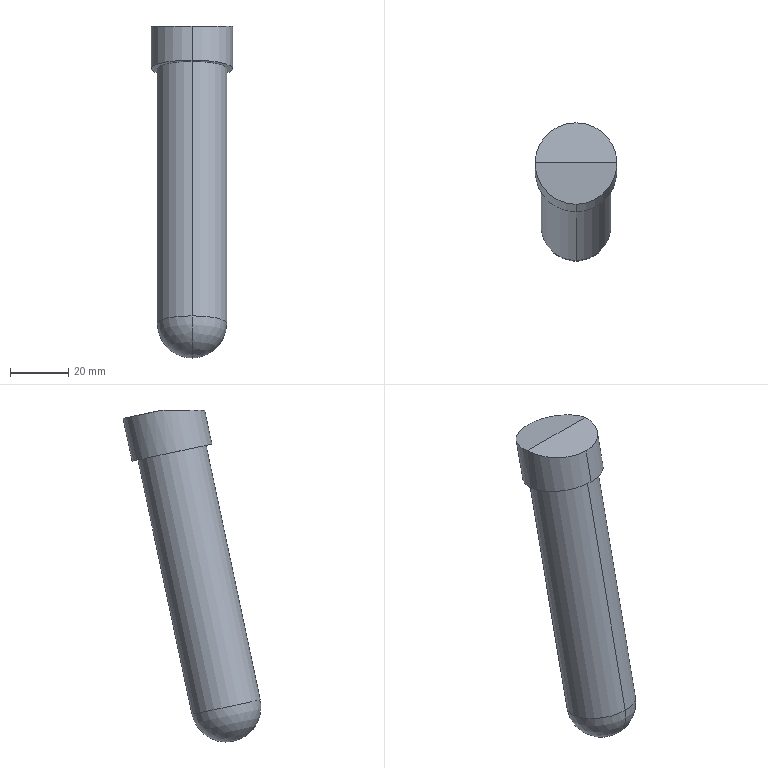Part | Creo | 1 solid | 9 faces | box 28.1 x 47.494 x 114.331 mm | volume 53070 mm3 | cylinder 4 | plane 3 | sphere 2 | commonest cylinder face diameters 24 x2 28.1 x2
STEP:
#1=CARTESIAN_POINT('',(110.,-266.619,89.579));
#2=VERTEX_POINT('',#1);
#3=CARTESIAN_POINT('',(95.95,-280.362,92.5));
#4=VERTEX_POINT('',#3);
#5=CARTESIAN_POINT('',(110.,-280.362,92.5));
#6=DIRECTION('',(0.,0.2079,0.9781));
#7=DIRECTION('',(0.,0.9781,-0.2079));
#8=AXIS2_PLACEMENT_3D('',#5,#6,#7);
#9=CIRCLE('',#8,14.05);
#10=EDGE_CURVE('',#2,#4,#9,.T.);
#11=ORIENTED_EDGE('',*,*,#10,.F.);
#12=CARTESIAN_POINT('',(124.05,-280.362,92.5));
#13=VERTEX_POINT('',#12);
#14=CARTESIAN_POINT('',(110.,-280.362,92.5));
#15=DIRECTION('',(0.,0.2079,0.9781));
#16=DIRECTION('',(1.,0.,0.));
#17=AXIS2_PLACEMENT_3D('',#14,#15,#16);
#18=CIRCLE('',#17,14.05);
#19=EDGE_CURVE('',#13,#2,#18,.T.);
#20=ORIENTED_EDGE('',*,*,#19,.F.);
#21=CARTESIAN_POINT('',(95.95,-280.362,92.5));
#22=DIRECTION('',(1.,0.,0.));
#23=VECTOR('',#22,28.1);
#24=LINE('',#21,#23);
#25=EDGE_CURVE('',#4,#13,#24,.T.);
#26=ORIENTED_EDGE('',*,*,#25,.F.);
#27=EDGE_LOOP('',(#11,#20,#26));
#28=FACE_OUTER_BOUND('',#27,.F.);
#29=CARTESIAN_POINT('',(110.,-280.362,92.5));
#30=DIRECTION('',(0.,0.2079,0.9781));
#31=DIRECTION('',(0.,-0.9781,0.2079));
#32=AXIS2_PLACEMENT_3D('',#29,#30,#31);
#33=PLANE('',#32);
#34=ADVANCED_FACE('',(#28),#33,.T.);
#35=CARTESIAN_POINT('',(110.,-297.224,80.749));
#36=VERTEX_POINT('',#35);
#37=CARTESIAN_POINT('',(110.,-269.738,74.907));
#38=VERTEX_POINT('',#37);
#39=CARTESIAN_POINT('',(110.,-283.481,77.828));
#40=DIRECTION('',(0.,-0.2079,-0.9781));
#41=DIRECTION('',(0.,-0.9781,0.2079));
#42=AXIS2_PLACEMENT_3D('',#39,#40,#41);
#43=CIRCLE('',#42,14.05);
#44=EDGE_CURVE('',#36,#38,#43,.T.);
#45=ORIENTED_EDGE('',*,*,#44,.T.);
#46=CARTESIAN_POINT('',(110.,-266.619,89.579));
#47=DIRECTION('',(0.,-0.2079,-0.9781));
#48=VECTOR('',#47,15.);
#49=LINE('',#46,#48);
#50=EDGE_CURVE('',#2,#38,#49,.T.);
#51=ORIENTED_EDGE('',*,*,#50,.F.);
#52=ORIENTED_EDGE('',*,*,#10,.T.);
#53=CARTESIAN_POINT('',(110.,-294.726,92.5));
#54=VERTEX_POINT('',#53);
#55=CARTESIAN_POINT('',(110.,-294.726,92.5));
#56=CARTESIAN_POINT('',(109.185,-294.726,92.5));
#57=CARTESIAN_POINT('',(107.581,-294.584,92.5));
#58=CARTESIAN_POINT('',(105.216,-293.946,92.5));
#59=CARTESIAN_POINT('',(102.983,-292.89,92.5));
#60=CARTESIAN_POINT('',(100.982,-291.47,92.5));
#61=CARTESIAN_POINT('',(99.234,-289.706,92.5));
#62=CARTESIAN_POINT('',(97.802,-287.636,92.5));
#63=CARTESIAN_POINT('',(96.753,-285.365,92.5));
#64=CARTESIAN_POINT('',(96.099,-282.91,92.5));
#65=CARTESIAN_POINT('',(95.95,-281.224,92.5));
#66=CARTESIAN_POINT('',(95.95,-280.362,92.5));
#67=B_SPLINE_CURVE_WITH_KNOTS('',3,(#55,#56,#57,#58,#59,#60,#61,#62,#63,#64,#65,#66),.UNSPECIFIED.,.F.,.F.,(4,1,1,1,1,1,1,1,1,4),(0.,0.1111,0.2222,0.3333,0.4444,0.5556,0.6667,0.7778,0.8889,1.),.UNSPECIFIED.);
#68=EDGE_CURVE('',#54,#4,#67,.T.);
#69=ORIENTED_EDGE('',*,*,#68,.F.);
#70=CARTESIAN_POINT('',(110.,-294.726,92.5));
#71=DIRECTION('',(0.,-0.2079,-0.9781));
#72=VECTOR('',#71,12.014);
#73=LINE('',#70,#72);
#74=EDGE_CURVE('',#54,#36,#73,.T.);
#75=ORIENTED_EDGE('',*,*,#74,.T.);
#76=EDGE_LOOP('',(#45,#51,#52,#69,#75));
#77=FACE_OUTER_BOUND('',#76,.F.);
#78=CARTESIAN_POINT('',(110.,-280.362,92.5));
#79=DIRECTION('',(0.,-0.2079,-0.9781));
#80=DIRECTION('',(0.,0.9781,-0.2079));
#81=AXIS2_PLACEMENT_3D('',#78,#79,#80);
#82=CYLINDRICAL_SURFACE('',#81,14.05);
#83=ADVANCED_FACE('',(#77),#82,.T.);
#84=ORIENTED_EDGE('',*,*,#44,.F.);
#85=CARTESIAN_POINT('',(110.,-283.481,77.828));
#86=DIRECTION('',(0.,-0.2079,-0.9781));
#87=DIRECTION('',(0.,0.9781,-0.2079));
#88=AXIS2_PLACEMENT_3D('',#85,#86,#87);
#89=CIRCLE('',#88,14.05);
#90=EDGE_CURVE('',#38,#36,#89,.T.);
#91=ORIENTED_EDGE('',*,*,#90,.F.);
#92=EDGE_LOOP('',(#84,#91));
#93=FACE_OUTER_BOUND('',#92,.F.);
#94=CARTESIAN_POINT('',(110.,-271.743,75.333));
#95=VERTEX_POINT('',#94);
#96=CARTESIAN_POINT('',(110.,-295.219,80.323));
#97=VERTEX_POINT('',#96);
#98=CARTESIAN_POINT('',(110.,-283.481,77.828));
#99=DIRECTION('',(0.,0.2079,0.9781));
#100=DIRECTION('',(0.,0.9781,-0.2079));
#101=AXIS2_PLACEMENT_3D('',#98,#99,#100);
#102=CIRCLE('',#101,12.);
#103=EDGE_CURVE('',#95,#97,#102,.T.);
#104=ORIENTED_EDGE('',*,*,#103,.F.);
#105=CARTESIAN_POINT('',(110.,-283.481,77.828));
#106=DIRECTION('',(0.,0.2079,0.9781));
#107=DIRECTION('',(0.,-0.9781,0.2079));
#108=AXIS2_PLACEMENT_3D('',#105,#106,#107);
#109=CIRCLE('',#108,12.);
#110=EDGE_CURVE('',#97,#95,#109,.T.);
#111=ORIENTED_EDGE('',*,*,#110,.F.);
#112=EDGE_LOOP('',(#104,#111));
#113=FACE_BOUND('',#112,.F.);
#114=CARTESIAN_POINT('',(110.,-283.481,77.828));
#115=DIRECTION('',(0.,-0.2079,-0.9781));
#116=DIRECTION('',(0.,0.9781,-0.2079));
#117=AXIS2_PLACEMENT_3D('',#114,#115,#116);
#118=PLANE('',#117);
#119=ADVANCED_FACE('',(#93,#113),#118,.T.);
#120=ORIENTED_EDGE('',*,*,#90,.T.);
#121=ORIENTED_EDGE('',*,*,#74,.F.);
#122=CARTESIAN_POINT('',(110.,-294.726,92.5));
#123=CARTESIAN_POINT('',(110.736,-294.726,92.5));
#124=CARTESIAN_POINT('',(112.185,-294.61,92.5));
#125=CARTESIAN_POINT('',(114.317,-294.092,92.5));
#126=CARTESIAN_POINT('',(116.337,-293.247,92.5));
#127=CARTESIAN_POINT('',(118.215,-292.088,92.5));
#128=CARTESIAN_POINT('',(119.908,-290.63,92.5));
#129=CARTESIAN_POINT('',(121.355,-288.921,92.5));
#130=CARTESIAN_POINT('',(122.521,-287.008,92.5));
#131=CARTESIAN_POINT('',(123.393,-284.901,92.5));
#132=CARTESIAN_POINT('',(123.929,-282.664,92.5));
#133=CARTESIAN_POINT('',(124.05,-281.138,92.5));
#134=CARTESIAN_POINT('',(124.05,-280.362,92.5));
#135=B_SPLINE_CURVE_WITH_KNOTS('',3,(#122,#123,#124,#125,#126,#127,#128,#129,#130,#131,#132,#133,#134),.UNSPECIFIED.,.F.,.F.,(4,1,1,1,1,1,1,1,1,1,4),(0.,0.1,0.2,0.3,0.4,0.5,0.6,0.7,0.8,0.9,1.),.UNSPECIFIED.);
#136=EDGE_CURVE('',#54,#13,#135,.T.);
#137=ORIENTED_EDGE('',*,*,#136,.T.);
#138=ORIENTED_EDGE('',*,*,#19,.T.);
#139=ORIENTED_EDGE('',*,*,#50,.T.);
#140=EDGE_LOOP('',(#120,#121,#137,#138,#139));
#141=FACE_OUTER_BOUND('',#140,.F.);
#142=CARTESIAN_POINT('',(110.,-280.362,92.5));
#143=DIRECTION('',(0.,-0.2079,-0.9781));
#144=DIRECTION('',(0.,0.9781,-0.2079));
#145=AXIS2_PLACEMENT_3D('',#142,#143,#144);
#146=CYLINDRICAL_SURFACE('',#145,14.05);
#147=ADVANCED_FACE('',(#141),#146,.T.);
#148=ORIENTED_EDGE('',*,*,#136,.F.);
#149=ORIENTED_EDGE('',*,*,#68,.T.);
#150=ORIENTED_EDGE('',*,*,#25,.T.);
#151=EDGE_LOOP('',(#148,#149,#150));
#152=FACE_OUTER_BOUND('',#151,.F.);
#153=CARTESIAN_POINT('',(390.,-289.362,92.5));
#154=DIRECTION('',(0.,0.,1.));
#155=DIRECTION('',(0.,1.,0.));
#156=AXIS2_PLACEMENT_3D('',#153,#154,#155);
#157=PLANE('',#156);
#158=ADVANCED_FACE('',(#152),#157,.T.);
#159=CARTESIAN_POINT('',(110.,-313.851,-7.336));
#160=VERTEX_POINT('',#159);
#161=CARTESIAN_POINT('',(110.,-290.376,-12.326));
#162=VERTEX_POINT('',#161);
#163=CARTESIAN_POINT('',(110.,-302.113,-9.831));
#164=DIRECTION('',(0.,-0.2079,-0.9781));
#165=DIRECTION('',(0.,-0.9781,0.2079));
#166=AXIS2_PLACEMENT_3D('',#163,#164,#165);
#167=CIRCLE('',#166,12.);
#168=EDGE_CURVE('',#160,#162,#167,.T.);
#169=ORIENTED_EDGE('',*,*,#168,.T.);
#170=CARTESIAN_POINT('',(110.,-271.743,75.333));
#171=DIRECTION('',(0.,-0.2079,-0.9781));
#172=VECTOR('',#171,89.617);
#173=LINE('',#170,#172);
#174=EDGE_CURVE('',#95,#162,#173,.T.);
#175=ORIENTED_EDGE('',*,*,#174,.F.);
#176=ORIENTED_EDGE('',*,*,#103,.T.);
#177=CARTESIAN_POINT('',(110.,-295.219,80.323));
#178=DIRECTION('',(0.,-0.2079,-0.9781));
#179=VECTOR('',#178,89.617);
#180=LINE('',#177,#179);
#181=EDGE_CURVE('',#97,#160,#180,.T.);
#182=ORIENTED_EDGE('',*,*,#181,.T.);
#183=EDGE_LOOP('',(#169,#175,#176,#182));
#184=FACE_OUTER_BOUND('',#183,.F.);
#185=CARTESIAN_POINT('',(110.,-284.119,74.828));
#186=DIRECTION('',(0.,-0.2079,-0.9781));
#187=DIRECTION('',(0.,0.9781,-0.2079));
#188=AXIS2_PLACEMENT_3D('',#185,#186,#187);
#189=CYLINDRICAL_SURFACE('',#188,12.);
#190=ADVANCED_FACE('',(#184),#189,.T.);
#191=ORIENTED_EDGE('',*,*,#168,.F.);
#192=CARTESIAN_POINT('',(110.,-304.608,-21.569));
#193=VERTEX_POINT('',#192);
#194=CARTESIAN_POINT('',(110.,-302.113,-9.831));
#195=DIRECTION('',(1.,0.,0.));
#196=DIRECTION('',(0.,-0.9781,0.2079));
#197=AXIS2_PLACEMENT_3D('',#194,#195,#196);
#198=CIRCLE('',#197,12.);
#199=EDGE_CURVE('',#160,#193,#198,.T.);
#200=ORIENTED_EDGE('',*,*,#199,.T.);
#201=CARTESIAN_POINT('',(110.,-302.113,-9.831));
#202=DIRECTION('',(-1.,0.,0.));
#203=DIRECTION('',(0.,0.9781,-0.2079));
#204=AXIS2_PLACEMENT_3D('',#201,#202,#203);
#205=CIRCLE('',#204,12.);
#206=EDGE_CURVE('',#162,#193,#205,.T.);
#207=ORIENTED_EDGE('',*,*,#206,.F.);
#208=EDGE_LOOP('',(#191,#200,#207));
#209=FACE_OUTER_BOUND('',#208,.F.);
#210=CARTESIAN_POINT('',(110.,-302.113,-9.831));
#211=DIRECTION('',(0.,-0.2079,-0.9781));
#212=DIRECTION('',(0.,0.9781,-0.2079));
#213=AXIS2_PLACEMENT_3D('',#210,#211,#212);
#214=SPHERICAL_SURFACE('',#213,12.);
#215=ADVANCED_FACE('',(#209),#214,.T.);
#216=CARTESIAN_POINT('',(110.,-302.113,-9.831));
#217=DIRECTION('',(0.,-0.2079,-0.9781));
#218=DIRECTION('',(0.,0.9781,-0.2079));
#219=AXIS2_PLACEMENT_3D('',#216,#217,#218);
#220=CIRCLE('',#219,12.);
#221=EDGE_CURVE('',#162,#160,#220,.T.);
#222=ORIENTED_EDGE('',*,*,#221,.F.);
#223=ORIENTED_EDGE('',*,*,#206,.T.);
#224=ORIENTED_EDGE('',*,*,#199,.F.);
#225=EDGE_LOOP('',(#222,#223,#224));
#226=FACE_OUTER_BOUND('',#225,.F.);
#227=CARTESIAN_POINT('',(110.,-302.113,-9.831));
#228=DIRECTION('',(0.,-0.2079,-0.9781));
#229=DIRECTION('',(0.,0.9781,-0.2079));
#230=AXIS2_PLACEMENT_3D('',#227,#228,#229);
#231=SPHERICAL_SURFACE('',#230,12.);
#232=ADVANCED_FACE('',(#226),#231,.T.);
#233=ORIENTED_EDGE('',*,*,#221,.T.);
#234=ORIENTED_EDGE('',*,*,#181,.F.);
#235=ORIENTED_EDGE('',*,*,#110,.T.);
#236=ORIENTED_EDGE('',*,*,#174,.T.);
#237=EDGE_LOOP('',(#233,#234,#235,#236));
#238=FACE_OUTER_BOUND('',#237,.F.);
#239=CARTESIAN_POINT('',(110.,-284.119,74.828));
#240=DIRECTION('',(0.,-0.2079,-0.9781));
#241=DIRECTION('',(0.,0.9781,-0.2079));
#242=AXIS2_PLACEMENT_3D('',#239,#240,#241);
#243=CYLINDRICAL_SURFACE('',#242,12.);
#244=ADVANCED_FACE('',(#238),#243,.T.);
#245=CLOSED_SHELL('',(#34,#83,#119,#147,#158,#190,#215,#232,#244));
#246=MANIFOLD_SOLID_BREP('',#245);
#247=(LENGTH_UNIT()NAMED_UNIT(*)SI_UNIT(.MILLI.,.METRE.));
#248=UNCERTAINTY_MEASURE_WITH_UNIT(LENGTH_MEASURE(0.01296),#247,'','');
#249=(NAMED_UNIT(*)PLANE_ANGLE_UNIT()SI_UNIT($,.RADIAN.));
#250=PLANE_ANGLE_MEASURE_WITH_UNIT(PLANE_ANGLE_MEASURE(0.01745),#249);
#251=(CONVERSION_BASED_UNIT('DEGREE',#250)NAMED_UNIT(*)PLANE_ANGLE_UNIT());
#252=(NAMED_UNIT(*)SI_UNIT($,.STERADIAN.)SOLID_ANGLE_UNIT());
#253=(GEOMETRIC_REPRESENTATION_CONTEXT(3)GLOBAL_UNCERTAINTY_ASSIGNED_CONTEXT((#248))GLOBAL_UNIT_ASSIGNED_CONTEXT((#247,#251,#252))REPRESENTATION_CONTEXT('',''));
#254=ADVANCED_BREP_SHAPE_REPRESENTATION('',(#246),#253);